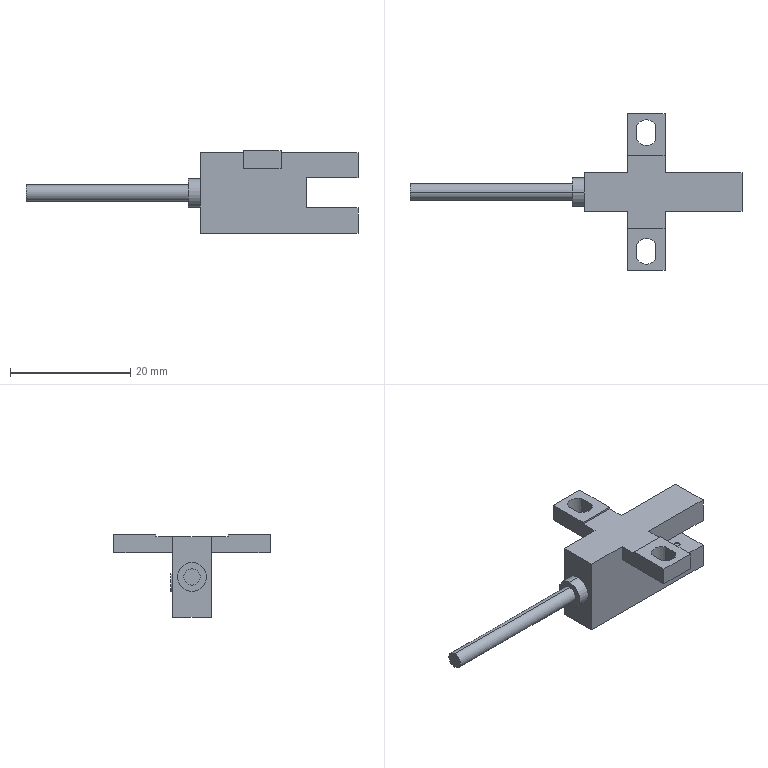Part | STEP file | PM-T44 | 1 solid | 45 faces | box 55.2 x 26 x 13.7 mm | volume 2450 mm3 | plane 31 | cylinder 14 | commonest cylinder face diameters 1 x4 3.6 x4 2.7 x2 3 x2 4.8 x2